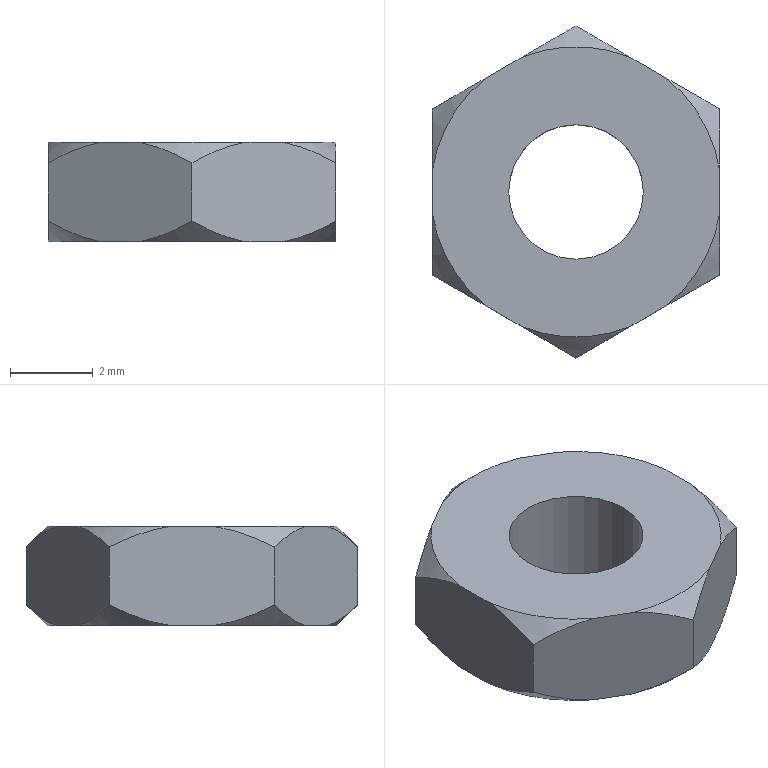Part | SolidWorks | features BaseBody 1 | 1 solid | 22 faces | box 6.928 x 8 x 2.4 mm | volume 78.962 mm3 | cone 12 | plane 8 | cylinder 2 | commonest cylinder face diameters 3.242 x2
STEP:
#1=CARTESIAN_POINT('',(1.396,-4.125,0.));
#2=VERTEX_POINT('',#1);
#3=CARTESIAN_POINT('',(4.638,-4.125,0.));
#4=VERTEX_POINT('',#3);
#5=CARTESIAN_POINT('',(3.017,-4.125,0.));
#6=DIRECTION('',(0.,0.,1.));
#7=DIRECTION('',(1.,0.,0.));
#8=AXIS2_PLACEMENT_3D('',#5,#6,#7);
#9=CIRCLE('',#8,1.621);
#10=EDGE_CURVE('',#2,#4,#9,.T.);
#11=ORIENTED_EDGE('',*,*,#10,.F.);
#12=CARTESIAN_POINT('',(1.396,-4.125,2.4));
#13=VERTEX_POINT('',#12);
#14=CARTESIAN_POINT('',(1.396,-4.125,-8.452));
#15=DIRECTION('',(0.,0.,1.));
#16=VECTOR('',#15,1000.);
#17=LINE('',#14,#16);
#18=EDGE_CURVE('',#2,#13,#17,.T.);
#19=ORIENTED_EDGE('',*,*,#18,.T.);
#20=CARTESIAN_POINT('',(4.638,-4.125,2.4));
#21=VERTEX_POINT('',#20);
#22=CARTESIAN_POINT('',(3.017,-4.125,2.4));
#23=DIRECTION('',(0.,0.,-1.));
#24=DIRECTION('',(1.,0.,0.));
#25=AXIS2_PLACEMENT_3D('',#22,#23,#24);
#26=CIRCLE('',#25,1.621);
#27=EDGE_CURVE('',#21,#13,#26,.T.);
#28=ORIENTED_EDGE('',*,*,#27,.F.);
#29=CARTESIAN_POINT('',(4.638,-4.125,-8.452));
#30=DIRECTION('',(0.,0.,1.));
#31=VECTOR('',#30,1000.);
#32=LINE('',#29,#31);
#33=EDGE_CURVE('',#4,#21,#32,.T.);
#34=ORIENTED_EDGE('',*,*,#33,.F.);
#35=EDGE_LOOP('',(#11,#19,#28,#34));
#36=FACE_OUTER_BOUND('',#35,.T.);
#37=CARTESIAN_POINT('',(3.017,-4.125,-8.452));
#38=DIRECTION('',(0.,0.,1.));
#39=DIRECTION('',(1.,0.,0.));
#40=AXIS2_PLACEMENT_3D('',#37,#38,#39);
#41=CYLINDRICAL_SURFACE('',#40,1.621);
#42=ADVANCED_FACE('',(#36),#41,.F.);
#43=CARTESIAN_POINT('',(3.017,-4.125,0.));
#44=DIRECTION('',(0.,0.,1.));
#45=DIRECTION('',(1.,0.,0.));
#46=AXIS2_PLACEMENT_3D('',#43,#44,#45);
#47=CIRCLE('',#46,1.621);
#48=EDGE_CURVE('',#4,#2,#47,.T.);
#49=ORIENTED_EDGE('',*,*,#48,.T.);
#50=ORIENTED_EDGE('',*,*,#10,.T.);
#51=EDGE_LOOP('',(#49,#50));
#52=FACE_BOUND('',#51,.T.);
#53=CARTESIAN_POINT('',(6.481,-3.625,0.));
#54=VERTEX_POINT('',#53);
#55=CARTESIAN_POINT('',(6.481,-4.625,0.));
#56=VERTEX_POINT('',#55);
#57=CARTESIAN_POINT('',(6.481,-4.125,0.));
#58=DIRECTION('',(0.,-1.,0.));
#59=VECTOR('',#58,1000.);
#60=LINE('',#57,#59);
#61=EDGE_CURVE('',#54,#56,#60,.T.);
#62=ORIENTED_EDGE('',*,*,#61,.T.);
#63=CARTESIAN_POINT('',(5.182,-6.875,0.));
#64=VERTEX_POINT('',#63);
#65=CARTESIAN_POINT('',(3.017,-4.125,0.));
#66=DIRECTION('',(0.,0.,-1.));
#67=DIRECTION('',(1.,0.,0.));
#68=AXIS2_PLACEMENT_3D('',#65,#66,#67);
#69=CIRCLE('',#68,3.5);
#70=EDGE_CURVE('',#56,#64,#69,.T.);
#71=ORIENTED_EDGE('',*,*,#70,.T.);
#72=CARTESIAN_POINT('',(4.316,-7.375,0.));
#73=VERTEX_POINT('',#72);
#74=CARTESIAN_POINT('',(5.182,-6.875,0.));
#75=DIRECTION('',(-0.866,-0.5,0.));
#76=VECTOR('',#75,1000.);
#77=LINE('',#74,#76);
#78=EDGE_CURVE('',#64,#73,#77,.T.);
#79=ORIENTED_EDGE('',*,*,#78,.T.);
#80=CARTESIAN_POINT('',(1.718,-7.375,0.));
#81=VERTEX_POINT('',#80);
#82=CARTESIAN_POINT('',(3.017,-4.125,0.));
#83=DIRECTION('',(0.,0.,-1.));
#84=DIRECTION('',(1.,0.,0.));
#85=AXIS2_PLACEMENT_3D('',#82,#83,#84);
#86=CIRCLE('',#85,3.5);
#87=EDGE_CURVE('',#73,#81,#86,.T.);
#88=ORIENTED_EDGE('',*,*,#87,.T.);
#89=CARTESIAN_POINT('',(0.8521,-6.875,0.));
#90=VERTEX_POINT('',#89);
#91=CARTESIAN_POINT('',(1.718,-7.375,0.));
#92=DIRECTION('',(-0.866,0.5,0.));
#93=VECTOR('',#92,1000.);
#94=LINE('',#91,#93);
#95=EDGE_CURVE('',#81,#90,#94,.T.);
#96=ORIENTED_EDGE('',*,*,#95,.T.);
#97=CARTESIAN_POINT('',(-0.447,-4.625,0.));
#98=VERTEX_POINT('',#97);
#99=CARTESIAN_POINT('',(3.017,-4.125,0.));
#100=DIRECTION('',(0.,0.,-1.));
#101=DIRECTION('',(1.,0.,0.));
#102=AXIS2_PLACEMENT_3D('',#99,#100,#101);
#103=CIRCLE('',#102,3.5);
#104=EDGE_CURVE('',#90,#98,#103,.T.);
#105=ORIENTED_EDGE('',*,*,#104,.T.);
#106=CARTESIAN_POINT('',(-0.447,-3.625,0.));
#107=VERTEX_POINT('',#106);
#108=CARTESIAN_POINT('',(-0.447,-4.125,0.));
#109=DIRECTION('',(0.,1.,0.));
#110=VECTOR('',#109,1000.);
#111=LINE('',#108,#110);
#112=EDGE_CURVE('',#98,#107,#111,.T.);
#113=ORIENTED_EDGE('',*,*,#112,.T.);
#114=CARTESIAN_POINT('',(0.8521,-1.375,0.));
#115=VERTEX_POINT('',#114);
#116=CARTESIAN_POINT('',(3.017,-4.125,0.));
#117=DIRECTION('',(0.,0.,-1.));
#118=DIRECTION('',(1.,0.,0.));
#119=AXIS2_PLACEMENT_3D('',#116,#117,#118);
#120=CIRCLE('',#119,3.5);
#121=EDGE_CURVE('',#107,#115,#120,.T.);
#122=ORIENTED_EDGE('',*,*,#121,.T.);
#123=CARTESIAN_POINT('',(1.718,-0.8753,0.));
#124=VERTEX_POINT('',#123);
#125=CARTESIAN_POINT('',(0.8521,-1.375,0.));
#126=DIRECTION('',(0.866,0.5,0.));
#127=VECTOR('',#126,1000.);
#128=LINE('',#125,#127);
#129=EDGE_CURVE('',#115,#124,#128,.T.);
#130=ORIENTED_EDGE('',*,*,#129,.T.);
#131=CARTESIAN_POINT('',(4.316,-0.8753,0.));
#132=VERTEX_POINT('',#131);
#133=CARTESIAN_POINT('',(3.017,-4.125,0.));
#134=DIRECTION('',(0.,0.,-1.));
#135=DIRECTION('',(1.,0.,0.));
#136=AXIS2_PLACEMENT_3D('',#133,#134,#135);
#137=CIRCLE('',#136,3.5);
#138=EDGE_CURVE('',#124,#132,#137,.T.);
#139=ORIENTED_EDGE('',*,*,#138,.T.);
#140=CARTESIAN_POINT('',(5.182,-1.375,0.));
#141=VERTEX_POINT('',#140);
#142=CARTESIAN_POINT('',(4.316,-0.8753,0.));
#143=DIRECTION('',(0.866,-0.5,0.));
#144=VECTOR('',#143,1000.);
#145=LINE('',#142,#144);
#146=EDGE_CURVE('',#132,#141,#145,.T.);
#147=ORIENTED_EDGE('',*,*,#146,.T.);
#148=CARTESIAN_POINT('',(3.017,-4.125,0.));
#149=DIRECTION('',(0.,0.,-1.));
#150=DIRECTION('',(1.,0.,0.));
#151=AXIS2_PLACEMENT_3D('',#148,#149,#150);
#152=CIRCLE('',#151,3.5);
#153=EDGE_CURVE('',#141,#54,#152,.T.);
#154=ORIENTED_EDGE('',*,*,#153,.T.);
#155=EDGE_LOOP('',(#62,#71,#79,#88,#96,#105,#113,#122,#130,#139,#147,#154));
#156=FACE_OUTER_BOUND('',#155,.T.);
#157=CARTESIAN_POINT('',(3.017,-4.125,0.));
#158=DIRECTION('',(0.,0.,-1.));
#159=DIRECTION('',(-1.,0.,0.));
#160=AXIS2_PLACEMENT_3D('',#157,#158,#159);
#161=PLANE('',#160);
#162=ADVANCED_FACE('',(#52,#156),#161,.T.);
#163=ORIENTED_EDGE('',*,*,#18,.F.);
#164=ORIENTED_EDGE('',*,*,#48,.F.);
#165=ORIENTED_EDGE('',*,*,#33,.T.);
#166=CARTESIAN_POINT('',(3.017,-4.125,2.4));
#167=DIRECTION('',(0.,0.,-1.));
#168=DIRECTION('',(1.,0.,0.));
#169=AXIS2_PLACEMENT_3D('',#166,#167,#168);
#170=CIRCLE('',#169,1.621);
#171=EDGE_CURVE('',#13,#21,#170,.T.);
#172=ORIENTED_EDGE('',*,*,#171,.F.);
#173=EDGE_LOOP('',(#163,#164,#165,#172));
#174=FACE_OUTER_BOUND('',#173,.T.);
#175=CARTESIAN_POINT('',(3.017,-4.125,-8.452));
#176=DIRECTION('',(0.,0.,1.));
#177=DIRECTION('',(1.,0.,0.));
#178=AXIS2_PLACEMENT_3D('',#175,#176,#177);
#179=CYLINDRICAL_SURFACE('',#178,1.621);
#180=ADVANCED_FACE('',(#174),#179,.F.);
#181=ORIENTED_EDGE('',*,*,#70,.F.);
#182=CARTESIAN_POINT('',(6.481,-6.125,0.5));
#183=VERTEX_POINT('',#182);
#184=CARTESIAN_POINT('',(6.481,-4.625,0.));
#185=CARTESIAN_POINT('',(6.481,-5.156,0.07576));
#186=CARTESIAN_POINT('',(6.481,-5.649,0.2619));
#187=CARTESIAN_POINT('',(6.481,-6.125,0.5));
#188=B_SPLINE_CURVE_WITH_KNOTS('',3,(#184,#185,#186,#187),.UNSPECIFIED.,.F.,.F.,(4,4),(0.,0.001581),.UNSPECIFIED.);
#189=EDGE_CURVE('',#56,#183,#188,.T.);
#190=ORIENTED_EDGE('',*,*,#189,.T.);
#191=CARTESIAN_POINT('',(6.481,-6.125,0.5));
#192=CARTESIAN_POINT('',(6.069,-6.363,0.2619));
#193=CARTESIAN_POINT('',(5.641,-6.61,0.07576));
#194=CARTESIAN_POINT('',(5.182,-6.875,0.));
#195=B_SPLINE_CURVE_WITH_KNOTS('',3,(#191,#192,#193,#194),.UNSPECIFIED.,.F.,.F.,(4,4),(0.,0.001581),.UNSPECIFIED.);
#196=EDGE_CURVE('',#183,#64,#195,.T.);
#197=ORIENTED_EDGE('',*,*,#196,.T.);
#198=EDGE_LOOP('',(#181,#190,#197));
#199=FACE_OUTER_BOUND('',#198,.T.);
#200=CARTESIAN_POINT('',(3.017,-4.125,0.503));
#201=DIRECTION('',(0.,0.,1.));
#202=DIRECTION('',(1.,0.,0.));
#203=AXIS2_PLACEMENT_3D('',#200,#201,#202);
#204=CONICAL_SURFACE('',#203,4.003,0.7854);
#205=ADVANCED_FACE('',(#199),#204,.T.);
#206=CARTESIAN_POINT('',(6.481,-3.625,2.4));
#207=VERTEX_POINT('',#206);
#208=CARTESIAN_POINT('',(6.481,-2.125,1.9));
#209=VERTEX_POINT('',#208);
#210=CARTESIAN_POINT('',(6.481,-3.625,2.4));
#211=CARTESIAN_POINT('',(6.481,-3.095,2.324));
#212=CARTESIAN_POINT('',(6.481,-2.601,2.138));
#213=CARTESIAN_POINT('',(6.481,-2.125,1.9));
#214=B_SPLINE_CURVE_WITH_KNOTS('',3,(#210,#211,#212,#213),.UNSPECIFIED.,.F.,.F.,(4,4),(0.,0.001581),.UNSPECIFIED.);
#215=EDGE_CURVE('',#207,#209,#214,.T.);
#216=ORIENTED_EDGE('',*,*,#215,.F.);
#217=CARTESIAN_POINT('',(6.481,-4.625,2.4));
#218=VERTEX_POINT('',#217);
#219=CARTESIAN_POINT('',(6.481,-6.125,2.4));
#220=DIRECTION('',(0.,-1.,0.));
#221=VECTOR('',#220,1000.);
#222=LINE('',#219,#221);
#223=EDGE_CURVE('',#207,#218,#222,.T.);
#224=ORIENTED_EDGE('',*,*,#223,.T.);
#225=CARTESIAN_POINT('',(6.481,-6.125,1.9));
#226=VERTEX_POINT('',#225);
#227=CARTESIAN_POINT('',(6.481,-6.125,1.9));
#228=CARTESIAN_POINT('',(6.481,-5.649,2.138));
#229=CARTESIAN_POINT('',(6.481,-5.156,2.324));
#230=CARTESIAN_POINT('',(6.481,-4.625,2.4));
#231=B_SPLINE_CURVE_WITH_KNOTS('',3,(#227,#228,#229,#230),.UNSPECIFIED.,.F.,.F.,(4,4),(0.,0.001581),.UNSPECIFIED.);
#232=EDGE_CURVE('',#226,#218,#231,.T.);
#233=ORIENTED_EDGE('',*,*,#232,.F.);
#234=CARTESIAN_POINT('',(6.481,-6.125,2.4));
#235=DIRECTION('',(0.,0.,-1.));
#236=VECTOR('',#235,1000.);
#237=LINE('',#234,#236);
#238=EDGE_CURVE('',#226,#183,#237,.T.);
#239=ORIENTED_EDGE('',*,*,#238,.T.);
#240=ORIENTED_EDGE('',*,*,#189,.F.);
#241=ORIENTED_EDGE('',*,*,#61,.F.);
#242=CARTESIAN_POINT('',(6.481,-2.125,0.5));
#243=VERTEX_POINT('',#242);
#244=CARTESIAN_POINT('',(6.481,-3.625,0.));
#245=CARTESIAN_POINT('',(6.481,-3.095,0.07576));
#246=CARTESIAN_POINT('',(6.481,-2.601,0.2619));
#247=CARTESIAN_POINT('',(6.481,-2.125,0.5));
#248=B_SPLINE_CURVE_WITH_KNOTS('',3,(#244,#245,#246,#247),.UNSPECIFIED.,.F.,.F.,(4,4),(0.,0.001581),.UNSPECIFIED.);
#249=EDGE_CURVE('',#54,#243,#248,.T.);
#250=ORIENTED_EDGE('',*,*,#249,.T.);
#251=CARTESIAN_POINT('',(6.481,-2.125,2.4));
#252=DIRECTION('',(0.,0.,1.));
#253=VECTOR('',#252,1000.);
#254=LINE('',#251,#253);
#255=EDGE_CURVE('',#243,#209,#254,.T.);
#256=ORIENTED_EDGE('',*,*,#255,.T.);
#257=EDGE_LOOP('',(#216,#224,#233,#239,#240,#241,#250,#256));
#258=FACE_OUTER_BOUND('',#257,.T.);
#259=CARTESIAN_POINT('',(6.481,-6.125,2.4));
#260=DIRECTION('',(1.,0.,0.));
#261=DIRECTION('',(0.,0.,-1.));
#262=AXIS2_PLACEMENT_3D('',#259,#260,#261);
#263=PLANE('',#262);
#264=ADVANCED_FACE('',(#258),#263,.T.);
#265=ORIENTED_EDGE('',*,*,#153,.F.);
#266=CARTESIAN_POINT('',(5.182,-1.375,0.));
#267=CARTESIAN_POINT('',(5.641,-1.64,0.07576));
#268=CARTESIAN_POINT('',(6.069,-1.887,0.2619));
#269=CARTESIAN_POINT('',(6.481,-2.125,0.5));
#270=B_SPLINE_CURVE_WITH_KNOTS('',3,(#266,#267,#268,#269),.UNSPECIFIED.,.F.,.F.,(4,4),(0.,0.001581),.UNSPECIFIED.);
#271=EDGE_CURVE('',#141,#243,#270,.T.);
#272=ORIENTED_EDGE('',*,*,#271,.T.);
#273=ORIENTED_EDGE('',*,*,#249,.F.);
#274=EDGE_LOOP('',(#265,#272,#273));
#275=FACE_OUTER_BOUND('',#274,.T.);
#276=CARTESIAN_POINT('',(3.017,-4.125,0.503));
#277=DIRECTION('',(0.,0.,1.));
#278=DIRECTION('',(1.,0.,0.));
#279=AXIS2_PLACEMENT_3D('',#276,#277,#278);
#280=CONICAL_SURFACE('',#279,4.003,0.7854);
#281=ADVANCED_FACE('',(#275),#280,.T.);
#282=CARTESIAN_POINT('',(4.316,-0.8753,2.4));
#283=VERTEX_POINT('',#282);
#284=CARTESIAN_POINT('',(3.017,-0.1253,1.9));
#285=VERTEX_POINT('',#284);
#286=CARTESIAN_POINT('',(4.316,-0.8753,2.4));
#287=CARTESIAN_POINT('',(3.857,-0.6101,2.324));
#288=CARTESIAN_POINT('',(3.43,-0.3634,2.138));
#289=CARTESIAN_POINT('',(3.017,-0.1253,1.9));
#290=B_SPLINE_CURVE_WITH_KNOTS('',3,(#286,#287,#288,#289),.UNSPECIFIED.,.F.,.F.,(4,4),(0.,0.001581),.UNSPECIFIED.);
#291=EDGE_CURVE('',#283,#285,#290,.T.);
#292=ORIENTED_EDGE('',*,*,#291,.F.);
#293=CARTESIAN_POINT('',(5.182,-1.375,2.4));
#294=VERTEX_POINT('',#293);
#295=CARTESIAN_POINT('',(6.481,-2.125,2.4));
#296=DIRECTION('',(0.866,-0.5,0.));
#297=VECTOR('',#296,1000.);
#298=LINE('',#295,#297);
#299=EDGE_CURVE('',#283,#294,#298,.T.);
#300=ORIENTED_EDGE('',*,*,#299,.T.);
#301=CARTESIAN_POINT('',(6.481,-2.125,1.9));
#302=CARTESIAN_POINT('',(6.069,-1.887,2.138));
#303=CARTESIAN_POINT('',(5.641,-1.64,2.324));
#304=CARTESIAN_POINT('',(5.182,-1.375,2.4));
#305=B_SPLINE_CURVE_WITH_KNOTS('',3,(#301,#302,#303,#304),.UNSPECIFIED.,.F.,.F.,(4,4),(0.,0.001581),.UNSPECIFIED.);
#306=EDGE_CURVE('',#209,#294,#305,.T.);
#307=ORIENTED_EDGE('',*,*,#306,.F.);
#308=ORIENTED_EDGE('',*,*,#255,.F.);
#309=ORIENTED_EDGE('',*,*,#271,.F.);
#310=ORIENTED_EDGE('',*,*,#146,.F.);
#311=CARTESIAN_POINT('',(3.017,-0.1253,0.5));
#312=VERTEX_POINT('',#311);
#313=CARTESIAN_POINT('',(4.316,-0.8753,0.));
#314=CARTESIAN_POINT('',(3.857,-0.6101,0.07576));
#315=CARTESIAN_POINT('',(3.43,-0.3634,0.2619));
#316=CARTESIAN_POINT('',(3.017,-0.1253,0.5));
#317=B_SPLINE_CURVE_WITH_KNOTS('',3,(#313,#314,#315,#316),.UNSPECIFIED.,.F.,.F.,(4,4),(0.,0.001581),.UNSPECIFIED.);
#318=EDGE_CURVE('',#132,#312,#317,.T.);
#319=ORIENTED_EDGE('',*,*,#318,.T.);
#320=CARTESIAN_POINT('',(3.017,-0.1253,2.4));
#321=DIRECTION('',(0.,0.,1.));
#322=VECTOR('',#321,1000.);
#323=LINE('',#320,#322);
#324=EDGE_CURVE('',#312,#285,#323,.T.);
#325=ORIENTED_EDGE('',*,*,#324,.T.);
#326=EDGE_LOOP('',(#292,#300,#307,#308,#309,#310,#319,#325));
#327=FACE_OUTER_BOUND('',#326,.T.);
#328=CARTESIAN_POINT('',(6.481,-2.125,2.4));
#329=DIRECTION('',(0.5,0.866,0.));
#330=DIRECTION('',(-0.866,0.5,0.));
#331=AXIS2_PLACEMENT_3D('',#328,#329,#330);
#332=PLANE('',#331);
#333=ADVANCED_FACE('',(#327),#332,.T.);
#334=ORIENTED_EDGE('',*,*,#138,.F.);
#335=CARTESIAN_POINT('',(1.718,-0.8753,0.));
#336=CARTESIAN_POINT('',(2.177,-0.6101,0.07576));
#337=CARTESIAN_POINT('',(2.605,-0.3634,0.2619));
#338=CARTESIAN_POINT('',(3.017,-0.1253,0.5));
#339=B_SPLINE_CURVE_WITH_KNOTS('',3,(#335,#336,#337,#338),.UNSPECIFIED.,.F.,.F.,(4,4),(0.,0.001581),.UNSPECIFIED.);
#340=EDGE_CURVE('',#124,#312,#339,.T.);
#341=ORIENTED_EDGE('',*,*,#340,.T.);
#342=ORIENTED_EDGE('',*,*,#318,.F.);
#343=EDGE_LOOP('',(#334,#341,#342));
#344=FACE_OUTER_BOUND('',#343,.T.);
#345=CARTESIAN_POINT('',(3.017,-4.125,0.503));
#346=DIRECTION('',(0.,0.,1.));
#347=DIRECTION('',(1.,0.,0.));
#348=AXIS2_PLACEMENT_3D('',#345,#346,#347);
#349=CONICAL_SURFACE('',#348,4.003,0.7854);
#350=ADVANCED_FACE('',(#344),#349,.T.);
#351=CARTESIAN_POINT('',(0.8521,-1.375,2.4));
#352=VERTEX_POINT('',#351);
#353=CARTESIAN_POINT('',(-0.447,-2.125,1.9));
#354=VERTEX_POINT('',#353);
#355=CARTESIAN_POINT('',(0.8521,-1.375,2.4));
#356=CARTESIAN_POINT('',(0.3928,-1.64,2.324));
#357=CARTESIAN_POINT('',(-0.03458,-1.887,2.138));
#358=CARTESIAN_POINT('',(-0.447,-2.125,1.9));
#359=B_SPLINE_CURVE_WITH_KNOTS('',3,(#355,#356,#357,#358),.UNSPECIFIED.,.F.,.F.,(4,4),(0.,0.001581),.UNSPECIFIED.);
#360=EDGE_CURVE('',#352,#354,#359,.T.);
#361=ORIENTED_EDGE('',*,*,#360,.F.);
#362=CARTESIAN_POINT('',(1.718,-0.8753,2.4));
#363=VERTEX_POINT('',#362);
#364=CARTESIAN_POINT('',(3.017,-0.1253,2.4));
#365=DIRECTION('',(0.866,0.5,0.));
#366=VECTOR('',#365,1000.);
#367=LINE('',#364,#366);
#368=EDGE_CURVE('',#352,#363,#367,.T.);
#369=ORIENTED_EDGE('',*,*,#368,.T.);
#370=CARTESIAN_POINT('',(3.017,-0.1253,1.9));
#371=CARTESIAN_POINT('',(2.605,-0.3634,2.138));
#372=CARTESIAN_POINT('',(2.177,-0.6101,2.324));
#373=CARTESIAN_POINT('',(1.718,-0.8753,2.4));
#374=B_SPLINE_CURVE_WITH_KNOTS('',3,(#370,#371,#372,#373),.UNSPECIFIED.,.F.,.F.,(4,4),(0.,0.001581),.UNSPECIFIED.);
#375=EDGE_CURVE('',#285,#363,#374,.T.);
#376=ORIENTED_EDGE('',*,*,#375,.F.);
#377=ORIENTED_EDGE('',*,*,#324,.F.);
#378=ORIENTED_EDGE('',*,*,#340,.F.);
#379=ORIENTED_EDGE('',*,*,#129,.F.);
#380=CARTESIAN_POINT('',(-0.447,-2.125,0.5));
#381=VERTEX_POINT('',#380);
#382=CARTESIAN_POINT('',(0.8521,-1.375,0.));
#383=CARTESIAN_POINT('',(0.3928,-1.64,0.07576));
#384=CARTESIAN_POINT('',(-0.03458,-1.887,0.2619));
#385=CARTESIAN_POINT('',(-0.447,-2.125,0.5));
#386=B_SPLINE_CURVE_WITH_KNOTS('',3,(#382,#383,#384,#385),.UNSPECIFIED.,.F.,.F.,(4,4),(0.,0.001581),.UNSPECIFIED.);
#387=EDGE_CURVE('',#115,#381,#386,.T.);
#388=ORIENTED_EDGE('',*,*,#387,.T.);
#389=CARTESIAN_POINT('',(-0.447,-2.125,2.4));
#390=DIRECTION('',(0.,0.,1.));
#391=VECTOR('',#390,1000.);
#392=LINE('',#389,#391);
#393=EDGE_CURVE('',#381,#354,#392,.T.);
#394=ORIENTED_EDGE('',*,*,#393,.T.);
#395=EDGE_LOOP('',(#361,#369,#376,#377,#378,#379,#388,#394));
#396=FACE_OUTER_BOUND('',#395,.T.);
#397=CARTESIAN_POINT('',(3.017,-0.1253,2.4));
#398=DIRECTION('',(-0.5,0.866,0.));
#399=DIRECTION('',(-0.866,-0.5,0.));
#400=AXIS2_PLACEMENT_3D('',#397,#398,#399);
#401=PLANE('',#400);
#402=ADVANCED_FACE('',(#396),#401,.T.);
#403=ORIENTED_EDGE('',*,*,#387,.F.);
#404=ORIENTED_EDGE('',*,*,#121,.F.);
#405=CARTESIAN_POINT('',(-0.447,-3.625,0.));
#406=CARTESIAN_POINT('',(-0.447,-3.095,0.07576));
#407=CARTESIAN_POINT('',(-0.447,-2.601,0.2619));
#408=CARTESIAN_POINT('',(-0.447,-2.125,0.5));
#409=B_SPLINE_CURVE_WITH_KNOTS('',3,(#405,#406,#407,#408),.UNSPECIFIED.,.F.,.F.,(4,4),(0.,0.001581),.UNSPECIFIED.);
#410=EDGE_CURVE('',#107,#381,#409,.T.);
#411=ORIENTED_EDGE('',*,*,#410,.T.);
#412=EDGE_LOOP('',(#403,#404,#411));
#413=FACE_OUTER_BOUND('',#412,.T.);
#414=CARTESIAN_POINT('',(3.017,-4.125,0.503));
#415=DIRECTION('',(0.,0.,1.));
#416=DIRECTION('',(1.,0.,0.));
#417=AXIS2_PLACEMENT_3D('',#414,#415,#416);
#418=CONICAL_SURFACE('',#417,4.003,0.7854);
#419=ADVANCED_FACE('',(#413),#418,.T.);
#420=CARTESIAN_POINT('',(-0.447,-6.125,0.5));
#421=VERTEX_POINT('',#420);
#422=CARTESIAN_POINT('',(-0.447,-4.625,0.));
#423=CARTESIAN_POINT('',(-0.447,-5.156,0.07576));
#424=CARTESIAN_POINT('',(-0.447,-5.649,0.2619));
#425=CARTESIAN_POINT('',(-0.447,-6.125,0.5));
#426=B_SPLINE_CURVE_WITH_KNOTS('',3,(#422,#423,#424,#425),.UNSPECIFIED.,.F.,.F.,(4,4),(0.,0.001581),.UNSPECIFIED.);
#427=EDGE_CURVE('',#98,#421,#426,.T.);
#428=ORIENTED_EDGE('',*,*,#427,.T.);
#429=CARTESIAN_POINT('',(-0.447,-6.125,1.9));
#430=VERTEX_POINT('',#429);
#431=CARTESIAN_POINT('',(-0.447,-6.125,2.4));
#432=DIRECTION('',(0.,0.,1.));
#433=VECTOR('',#432,1000.);
#434=LINE('',#431,#433);
#435=EDGE_CURVE('',#421,#430,#434,.T.);
#436=ORIENTED_EDGE('',*,*,#435,.T.);
#437=CARTESIAN_POINT('',(-0.447,-4.625,2.4));
#438=VERTEX_POINT('',#437);
#439=CARTESIAN_POINT('',(-0.447,-4.625,2.4));
#440=CARTESIAN_POINT('',(-0.447,-5.156,2.324));
#441=CARTESIAN_POINT('',(-0.447,-5.649,2.138));
#442=CARTESIAN_POINT('',(-0.447,-6.125,1.9));
#443=B_SPLINE_CURVE_WITH_KNOTS('',3,(#439,#440,#441,#442),.UNSPECIFIED.,.F.,.F.,(4,4),(0.,0.001581),.UNSPECIFIED.);
#444=EDGE_CURVE('',#438,#430,#443,.T.);
#445=ORIENTED_EDGE('',*,*,#444,.F.);
#446=CARTESIAN_POINT('',(-0.447,-3.625,2.4));
#447=VERTEX_POINT('',#446);
#448=CARTESIAN_POINT('',(-0.447,-2.125,2.4));
#449=DIRECTION('',(0.,1.,0.));
#450=VECTOR('',#449,1000.);
#451=LINE('',#448,#450);
#452=EDGE_CURVE('',#438,#447,#451,.T.);
#453=ORIENTED_EDGE('',*,*,#452,.T.);
#454=CARTESIAN_POINT('',(-0.447,-2.125,1.9));
#455=CARTESIAN_POINT('',(-0.447,-2.601,2.138));
#456=CARTESIAN_POINT('',(-0.447,-3.095,2.324));
#457=CARTESIAN_POINT('',(-0.447,-3.625,2.4));
#458=B_SPLINE_CURVE_WITH_KNOTS('',3,(#454,#455,#456,#457),.UNSPECIFIED.,.F.,.F.,(4,4),(0.,0.001581),.UNSPECIFIED.);
#459=EDGE_CURVE('',#354,#447,#458,.T.);
#460=ORIENTED_EDGE('',*,*,#459,.F.);
#461=ORIENTED_EDGE('',*,*,#393,.F.);
#462=ORIENTED_EDGE('',*,*,#410,.F.);
#463=ORIENTED_EDGE('',*,*,#112,.F.);
#464=EDGE_LOOP('',(#428,#436,#445,#453,#460,#461,#462,#463));
#465=FACE_OUTER_BOUND('',#464,.T.);
#466=CARTESIAN_POINT('',(-0.447,-2.125,2.4));
#467=DIRECTION('',(-1.,0.,0.));
#468=DIRECTION('',(0.,0.,1.));
#469=AXIS2_PLACEMENT_3D('',#466,#467,#468);
#470=PLANE('',#469);
#471=ADVANCED_FACE('',(#465),#470,.T.);
#472=ORIENTED_EDGE('',*,*,#427,.F.);
#473=ORIENTED_EDGE('',*,*,#104,.F.);
#474=CARTESIAN_POINT('',(0.8521,-6.875,0.));
#475=CARTESIAN_POINT('',(0.3928,-6.61,0.07576));
#476=CARTESIAN_POINT('',(-0.03458,-6.363,0.2619));
#477=CARTESIAN_POINT('',(-0.447,-6.125,0.5));
#478=B_SPLINE_CURVE_WITH_KNOTS('',3,(#474,#475,#476,#477),.UNSPECIFIED.,.F.,.F.,(4,4),(0.,0.001581),.UNSPECIFIED.);
#479=EDGE_CURVE('',#90,#421,#478,.T.);
#480=ORIENTED_EDGE('',*,*,#479,.T.);
#481=EDGE_LOOP('',(#472,#473,#480));
#482=FACE_OUTER_BOUND('',#481,.T.);
#483=CARTESIAN_POINT('',(3.017,-4.125,0.503));
#484=DIRECTION('',(0.,0.,1.));
#485=DIRECTION('',(1.,0.,0.));
#486=AXIS2_PLACEMENT_3D('',#483,#484,#485);
#487=CONICAL_SURFACE('',#486,4.003,0.7854);
#488=ADVANCED_FACE('',(#482),#487,.T.);
#489=CARTESIAN_POINT('',(3.017,-8.125,0.5));
#490=VERTEX_POINT('',#489);
#491=CARTESIAN_POINT('',(1.718,-7.375,0.));
#492=CARTESIAN_POINT('',(2.177,-7.64,0.07576));
#493=CARTESIAN_POINT('',(2.605,-7.887,0.2619));
#494=CARTESIAN_POINT('',(3.017,-8.125,0.5));
#495=B_SPLINE_CURVE_WITH_KNOTS('',3,(#491,#492,#493,#494),.UNSPECIFIED.,.F.,.F.,(4,4),(0.,0.001581),.UNSPECIFIED.);
#496=EDGE_CURVE('',#81,#490,#495,.T.);
#497=ORIENTED_EDGE('',*,*,#496,.T.);
#498=CARTESIAN_POINT('',(3.017,-8.125,1.9));
#499=VERTEX_POINT('',#498);
#500=CARTESIAN_POINT('',(3.017,-8.125,2.4));
#501=DIRECTION('',(0.,0.,1.));
#502=VECTOR('',#501,1000.);
#503=LINE('',#500,#502);
#504=EDGE_CURVE('',#490,#499,#503,.T.);
#505=ORIENTED_EDGE('',*,*,#504,.T.);
#506=CARTESIAN_POINT('',(1.718,-7.375,2.4));
#507=VERTEX_POINT('',#506);
#508=CARTESIAN_POINT('',(1.718,-7.375,2.4));
#509=CARTESIAN_POINT('',(2.177,-7.64,2.324));
#510=CARTESIAN_POINT('',(2.605,-7.887,2.138));
#511=CARTESIAN_POINT('',(3.017,-8.125,1.9));
#512=B_SPLINE_CURVE_WITH_KNOTS('',3,(#508,#509,#510,#511),.UNSPECIFIED.,.F.,.F.,(4,4),(0.,0.001581),.UNSPECIFIED.);
#513=EDGE_CURVE('',#507,#499,#512,.T.);
#514=ORIENTED_EDGE('',*,*,#513,.F.);
#515=CARTESIAN_POINT('',(0.8521,-6.875,2.4));
#516=VERTEX_POINT('',#515);
#517=CARTESIAN_POINT('',(-0.447,-6.125,2.4));
#518=DIRECTION('',(-0.866,0.5,0.));
#519=VECTOR('',#518,1000.);
#520=LINE('',#517,#519);
#521=EDGE_CURVE('',#507,#516,#520,.T.);
#522=ORIENTED_EDGE('',*,*,#521,.T.);
#523=CARTESIAN_POINT('',(-0.447,-6.125,1.9));
#524=CARTESIAN_POINT('',(-0.03458,-6.363,2.138));
#525=CARTESIAN_POINT('',(0.3928,-6.61,2.324));
#526=CARTESIAN_POINT('',(0.8521,-6.875,2.4));
#527=B_SPLINE_CURVE_WITH_KNOTS('',3,(#523,#524,#525,#526),.UNSPECIFIED.,.F.,.F.,(4,4),(0.,0.001581),.UNSPECIFIED.);
#528=EDGE_CURVE('',#430,#516,#527,.T.);
#529=ORIENTED_EDGE('',*,*,#528,.F.);
#530=ORIENTED_EDGE('',*,*,#435,.F.);
#531=ORIENTED_EDGE('',*,*,#479,.F.);
#532=ORIENTED_EDGE('',*,*,#95,.F.);
#533=EDGE_LOOP('',(#497,#505,#514,#522,#529,#530,#531,#532));
#534=FACE_OUTER_BOUND('',#533,.T.);
#535=CARTESIAN_POINT('',(-0.447,-6.125,2.4));
#536=DIRECTION('',(-0.5,-0.866,0.));
#537=DIRECTION('',(0.866,-0.5,0.));
#538=AXIS2_PLACEMENT_3D('',#535,#536,#537);
#539=PLANE('',#538);
#540=ADVANCED_FACE('',(#534),#539,.T.);
#541=ORIENTED_EDGE('',*,*,#87,.F.);
#542=CARTESIAN_POINT('',(4.316,-7.375,0.));
#543=CARTESIAN_POINT('',(3.857,-7.64,0.07576));
#544=CARTESIAN_POINT('',(3.43,-7.887,0.2619));
#545=CARTESIAN_POINT('',(3.017,-8.125,0.5));
#546=B_SPLINE_CURVE_WITH_KNOTS('',3,(#542,#543,#544,#545),.UNSPECIFIED.,.F.,.F.,(4,4),(0.,0.001581),.UNSPECIFIED.);
#547=EDGE_CURVE('',#73,#490,#546,.T.);
#548=ORIENTED_EDGE('',*,*,#547,.T.);
#549=ORIENTED_EDGE('',*,*,#496,.F.);
#550=EDGE_LOOP('',(#541,#548,#549));
#551=FACE_OUTER_BOUND('',#550,.T.);
#552=CARTESIAN_POINT('',(3.017,-4.125,0.503));
#553=DIRECTION('',(0.,0.,1.));
#554=DIRECTION('',(1.,0.,0.));
#555=AXIS2_PLACEMENT_3D('',#552,#553,#554);
#556=CONICAL_SURFACE('',#555,4.003,0.7854);
#557=ADVANCED_FACE('',(#551),#556,.T.);
#558=ORIENTED_EDGE('',*,*,#196,.F.);
#559=ORIENTED_EDGE('',*,*,#238,.F.);
#560=CARTESIAN_POINT('',(5.182,-6.875,2.4));
#561=VERTEX_POINT('',#560);
#562=CARTESIAN_POINT('',(5.182,-6.875,2.4));
#563=CARTESIAN_POINT('',(5.641,-6.61,2.324));
#564=CARTESIAN_POINT('',(6.069,-6.363,2.138));
#565=CARTESIAN_POINT('',(6.481,-6.125,1.9));
#566=B_SPLINE_CURVE_WITH_KNOTS('',3,(#562,#563,#564,#565),.UNSPECIFIED.,.F.,.F.,(4,4),(0.,0.001581),.UNSPECIFIED.);
#567=EDGE_CURVE('',#561,#226,#566,.T.);
#568=ORIENTED_EDGE('',*,*,#567,.F.);
#569=CARTESIAN_POINT('',(4.316,-7.375,2.4));
#570=VERTEX_POINT('',#569);
#571=CARTESIAN_POINT('',(3.017,-8.125,2.4));
#572=DIRECTION('',(-0.866,-0.5,0.));
#573=VECTOR('',#572,1000.);
#574=LINE('',#571,#573);
#575=EDGE_CURVE('',#561,#570,#574,.T.);
#576=ORIENTED_EDGE('',*,*,#575,.T.);
#577=CARTESIAN_POINT('',(3.017,-8.125,1.9));
#578=CARTESIAN_POINT('',(3.43,-7.887,2.138));
#579=CARTESIAN_POINT('',(3.857,-7.64,2.324));
#580=CARTESIAN_POINT('',(4.316,-7.375,2.4));
#581=B_SPLINE_CURVE_WITH_KNOTS('',3,(#577,#578,#579,#580),.UNSPECIFIED.,.F.,.F.,(4,4),(0.,0.001581),.UNSPECIFIED.);
#582=EDGE_CURVE('',#499,#570,#581,.T.);
#583=ORIENTED_EDGE('',*,*,#582,.F.);
#584=ORIENTED_EDGE('',*,*,#504,.F.);
#585=ORIENTED_EDGE('',*,*,#547,.F.);
#586=ORIENTED_EDGE('',*,*,#78,.F.);
#587=EDGE_LOOP('',(#558,#559,#568,#576,#583,#584,#585,#586));
#588=FACE_OUTER_BOUND('',#587,.T.);
#589=CARTESIAN_POINT('',(3.017,-8.125,2.4));
#590=DIRECTION('',(0.5,-0.866,0.));
#591=DIRECTION('',(0.866,0.5,0.));
#592=AXIS2_PLACEMENT_3D('',#589,#590,#591);
#593=PLANE('',#592);
#594=ADVANCED_FACE('',(#588),#593,.T.);
#595=ORIENTED_EDGE('',*,*,#27,.T.);
#596=ORIENTED_EDGE('',*,*,#171,.T.);
#597=EDGE_LOOP('',(#595,#596));
#598=FACE_BOUND('',#597,.T.);
#599=CARTESIAN_POINT('',(3.017,-4.125,2.4));
#600=DIRECTION('',(0.,0.,-1.));
#601=DIRECTION('',(-1.,0.,0.));
#602=AXIS2_PLACEMENT_3D('',#599,#600,#601);
#603=CIRCLE('',#602,3.5);
#604=EDGE_CURVE('',#570,#507,#603,.T.);
#605=ORIENTED_EDGE('',*,*,#604,.F.);
#606=ORIENTED_EDGE('',*,*,#575,.F.);
#607=CARTESIAN_POINT('',(3.017,-4.125,2.4));
#608=DIRECTION('',(0.,0.,-1.));
#609=DIRECTION('',(-1.,0.,0.));
#610=AXIS2_PLACEMENT_3D('',#607,#608,#609);
#611=CIRCLE('',#610,3.5);
#612=EDGE_CURVE('',#218,#561,#611,.T.);
#613=ORIENTED_EDGE('',*,*,#612,.F.);
#614=ORIENTED_EDGE('',*,*,#223,.F.);
#615=CARTESIAN_POINT('',(3.017,-4.125,2.4));
#616=DIRECTION('',(0.,0.,-1.));
#617=DIRECTION('',(-1.,0.,0.));
#618=AXIS2_PLACEMENT_3D('',#615,#616,#617);
#619=CIRCLE('',#618,3.5);
#620=EDGE_CURVE('',#294,#207,#619,.T.);
#621=ORIENTED_EDGE('',*,*,#620,.F.);
#622=ORIENTED_EDGE('',*,*,#299,.F.);
#623=CARTESIAN_POINT('',(3.017,-4.125,2.4));
#624=DIRECTION('',(0.,0.,-1.));
#625=DIRECTION('',(-1.,0.,0.));
#626=AXIS2_PLACEMENT_3D('',#623,#624,#625);
#627=CIRCLE('',#626,3.5);
#628=EDGE_CURVE('',#363,#283,#627,.T.);
#629=ORIENTED_EDGE('',*,*,#628,.F.);
#630=ORIENTED_EDGE('',*,*,#368,.F.);
#631=CARTESIAN_POINT('',(3.017,-4.125,2.4));
#632=DIRECTION('',(0.,0.,-1.));
#633=DIRECTION('',(-1.,0.,0.));
#634=AXIS2_PLACEMENT_3D('',#631,#632,#633);
#635=CIRCLE('',#634,3.5);
#636=EDGE_CURVE('',#447,#352,#635,.T.);
#637=ORIENTED_EDGE('',*,*,#636,.F.);
#638=ORIENTED_EDGE('',*,*,#452,.F.);
#639=CARTESIAN_POINT('',(3.017,-4.125,2.4));
#640=DIRECTION('',(0.,0.,-1.));
#641=DIRECTION('',(-1.,0.,0.));
#642=AXIS2_PLACEMENT_3D('',#639,#640,#641);
#643=CIRCLE('',#642,3.5);
#644=EDGE_CURVE('',#516,#438,#643,.T.);
#645=ORIENTED_EDGE('',*,*,#644,.F.);
#646=ORIENTED_EDGE('',*,*,#521,.F.);
#647=EDGE_LOOP('',(#605,#606,#613,#614,#621,#622,#629,#630,#637,#638,#645,#646));
#648=FACE_OUTER_BOUND('',#647,.T.);
#649=CARTESIAN_POINT('',(3.017,-4.125,2.4));
#650=DIRECTION('',(0.,0.,-1.));
#651=DIRECTION('',(-1.,0.,0.));
#652=AXIS2_PLACEMENT_3D('',#649,#650,#651);
#653=PLANE('',#652);
#654=ADVANCED_FACE('',(#598,#648),#653,.F.);
#655=ORIENTED_EDGE('',*,*,#582,.T.);
#656=ORIENTED_EDGE('',*,*,#604,.T.);
#657=ORIENTED_EDGE('',*,*,#513,.T.);
#658=EDGE_LOOP('',(#655,#656,#657));
#659=FACE_OUTER_BOUND('',#658,.T.);
#660=CARTESIAN_POINT('',(3.017,-4.125,1.897));
#661=DIRECTION('',(0.,0.,-1.));
#662=DIRECTION('',(-1.,0.,0.));
#663=AXIS2_PLACEMENT_3D('',#660,#661,#662);
#664=CONICAL_SURFACE('',#663,4.003,0.7854);
#665=ADVANCED_FACE('',(#659),#664,.T.);
#666=ORIENTED_EDGE('',*,*,#232,.T.);
#667=ORIENTED_EDGE('',*,*,#612,.T.);
#668=ORIENTED_EDGE('',*,*,#567,.T.);
#669=EDGE_LOOP('',(#666,#667,#668));
#670=FACE_OUTER_BOUND('',#669,.T.);
#671=CARTESIAN_POINT('',(3.017,-4.125,1.897));
#672=DIRECTION('',(0.,0.,-1.));
#673=DIRECTION('',(-1.,0.,0.));
#674=AXIS2_PLACEMENT_3D('',#671,#672,#673);
#675=CONICAL_SURFACE('',#674,4.003,0.7854);
#676=ADVANCED_FACE('',(#670),#675,.T.);
#677=ORIENTED_EDGE('',*,*,#306,.T.);
#678=ORIENTED_EDGE('',*,*,#620,.T.);
#679=ORIENTED_EDGE('',*,*,#215,.T.);
#680=EDGE_LOOP('',(#677,#678,#679));
#681=FACE_OUTER_BOUND('',#680,.T.);
#682=CARTESIAN_POINT('',(3.017,-4.125,1.897));
#683=DIRECTION('',(0.,0.,-1.));
#684=DIRECTION('',(-1.,0.,0.));
#685=AXIS2_PLACEMENT_3D('',#682,#683,#684);
#686=CONICAL_SURFACE('',#685,4.003,0.7854);
#687=ADVANCED_FACE('',(#681),#686,.T.);
#688=ORIENTED_EDGE('',*,*,#375,.T.);
#689=ORIENTED_EDGE('',*,*,#628,.T.);
#690=ORIENTED_EDGE('',*,*,#291,.T.);
#691=EDGE_LOOP('',(#688,#689,#690));
#692=FACE_OUTER_BOUND('',#691,.T.);
#693=CARTESIAN_POINT('',(3.017,-4.125,1.897));
#694=DIRECTION('',(0.,0.,-1.));
#695=DIRECTION('',(-1.,0.,0.));
#696=AXIS2_PLACEMENT_3D('',#693,#694,#695);
#697=CONICAL_SURFACE('',#696,4.003,0.7854);
#698=ADVANCED_FACE('',(#692),#697,.T.);
#699=ORIENTED_EDGE('',*,*,#636,.T.);
#700=ORIENTED_EDGE('',*,*,#360,.T.);
#701=ORIENTED_EDGE('',*,*,#459,.T.);
#702=EDGE_LOOP('',(#699,#700,#701));
#703=FACE_OUTER_BOUND('',#702,.T.);
#704=CARTESIAN_POINT('',(3.017,-4.125,1.897));
#705=DIRECTION('',(0.,0.,-1.));
#706=DIRECTION('',(-1.,0.,0.));
#707=AXIS2_PLACEMENT_3D('',#704,#705,#706);
#708=CONICAL_SURFACE('',#707,4.003,0.7854);
#709=ADVANCED_FACE('',(#703),#708,.T.);
#710=ORIENTED_EDGE('',*,*,#644,.T.);
#711=ORIENTED_EDGE('',*,*,#444,.T.);
#712=ORIENTED_EDGE('',*,*,#528,.T.);
#713=EDGE_LOOP('',(#710,#711,#712));
#714=FACE_OUTER_BOUND('',#713,.T.);
#715=CARTESIAN_POINT('',(3.017,-4.125,1.897));
#716=DIRECTION('',(0.,0.,-1.));
#717=DIRECTION('',(-1.,0.,0.));
#718=AXIS2_PLACEMENT_3D('',#715,#716,#717);
#719=CONICAL_SURFACE('',#718,4.003,0.7854);
#720=ADVANCED_FACE('',(#714),#719,.T.);
#721=CLOSED_SHELL('',(#42,#162,#180,#205,#264,#281,#333,#350,#402,#419,#471,#488,#540,#557,#594,#654,#665,#676,#687,#698,#709,#720));
#722=MANIFOLD_SOLID_BREP('',#721);
#723=CARTESIAN_POINT('',(0.,0.,0.));
#724=DIRECTION('',(0.,0.,1.));
#725=DIRECTION('',(1.,0.,0.));
#726=AXIS2_PLACEMENT_3D('',#723,#724,#725);
#727=(LENGTH_UNIT()NAMED_UNIT(*)SI_UNIT(.MILLI.,.METRE.));
#728=UNCERTAINTY_MEASURE_WITH_UNIT(LENGTH_MEASURE(0.00001),#727,'','');
#729=(NAMED_UNIT(*)PLANE_ANGLE_UNIT()SI_UNIT($,.RADIAN.));
#730=(NAMED_UNIT(*)SI_UNIT($,.STERADIAN.)SOLID_ANGLE_UNIT());
#731=(GEOMETRIC_REPRESENTATION_CONTEXT(3)GLOBAL_UNCERTAINTY_ASSIGNED_CONTEXT((#728))GLOBAL_UNIT_ASSIGNED_CONTEXT((#727,#729,#730))REPRESENTATION_CONTEXT('',''));
#732=ADVANCED_BREP_SHAPE_REPRESENTATION('',(#722,#726),#731);